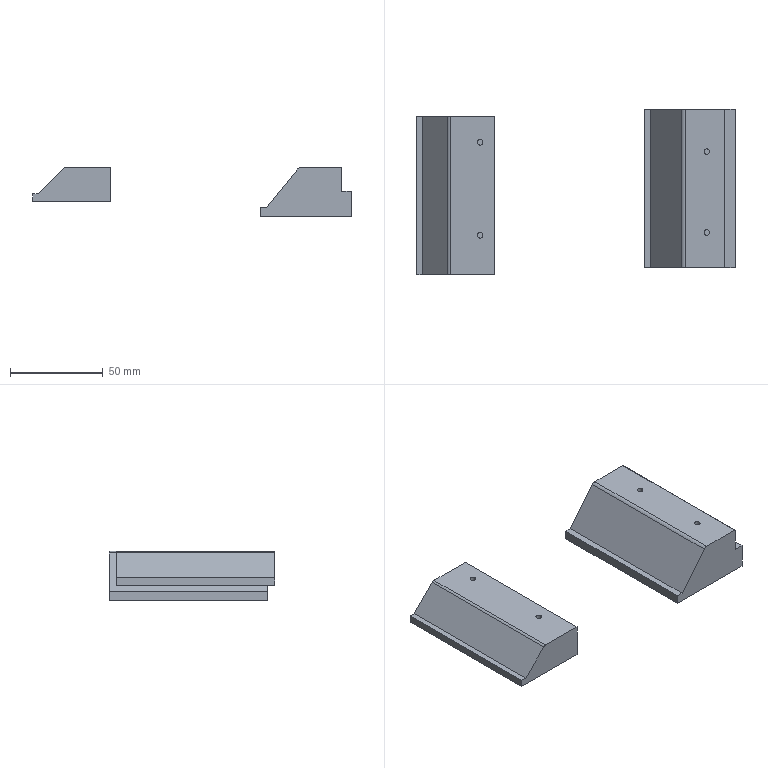NC program | NX | posted with a generic post | part box 171.319 x 88.841 x 26.598 mm
Whole program:
N10 G17 G21 G94 G90
(FLOOR_WALL_COPY_COPY , TOOL : D80)
N12 T19 M6
N14 G54
N16 G17 G0 G90 X-89.5 Y0. S6500 M3
N18 G43 Z30. H19
N20 Z9.
N22 G94 G1 Z6. F1500.
N24 X-84.5
N26 X84.5
N28 X89.5
N30 Z9.
N32 G0 Z30.
N34 X-89.5
N36 Z8.
N38 G1 Z5.
N40 X-84.5
N42 X84.5
N44 X89.5
N46 Z8.
N48 G0 Z30.
N50 X-89.5
N52 Z7.
N54 G1 Z4.
N56 X-84.5
N58 X84.5
N60 X89.5
N62 Z7.
N64 G0 Z30.
N66 X-89.5
N68 Z6.
N70 G1 Z3.
N72 X-84.5
N74 X84.5
N76 X89.5
N78 Z6.
N80 G0 Z30.
N82 X-89.5
N84 Z5.
N86 G1 Z2.
N88 X-84.5
N90 X84.5
N92 X89.5
N94 Z5.
N96 G0 Z30.
N98 X-89.5
N100 Z4.
N102 G1 Z1.
N104 X-84.5
N106 X84.5
N108 X89.5
N110 Z4.
N112 G0 Z30.
N114 X-89.5
N116 Z3.
N118 G1 Z0.
N120 X-84.5
N122 X84.5
N124 X89.5
N126 Z3.
N128 G0 Z30.
N130 M5
(PLANAR_MILL_COPY_COPY_COPY_COPY_COPY_COPY_1_COPY_1_COPY , TOOL : D6A45)
N132 T01 M6
N134 G54
N136 G17 G0 G90 X-1.27 Y23.1 S9500 M3
N138 G43 Z30. H1
N140 Z0.5
N142 G94 G1 Z-1. F1250.
N144 X-0.866 Y22.4
N146 G3 X0. Y21.9 R1.
N148 G1 X42.4
N150 G2 X43.4 Y20.9 R1.
N152 G1 Y-20.9
N154 G2 X42.4 Y-21.9 R1.
N156 G1 X-42.4
N158 G2 X-43.4 Y-20.9 R1.
N160 G1 Y20.9
N162 G2 X-42.4 Y21.9 R1.
N164 G1 X0.
N166 G3 X0.866 Y22.4 R1.
N168 G1 X1.27 Y23.1
N170 Z0.5
N172 G0 Z30.
N174 M5
N176 M2